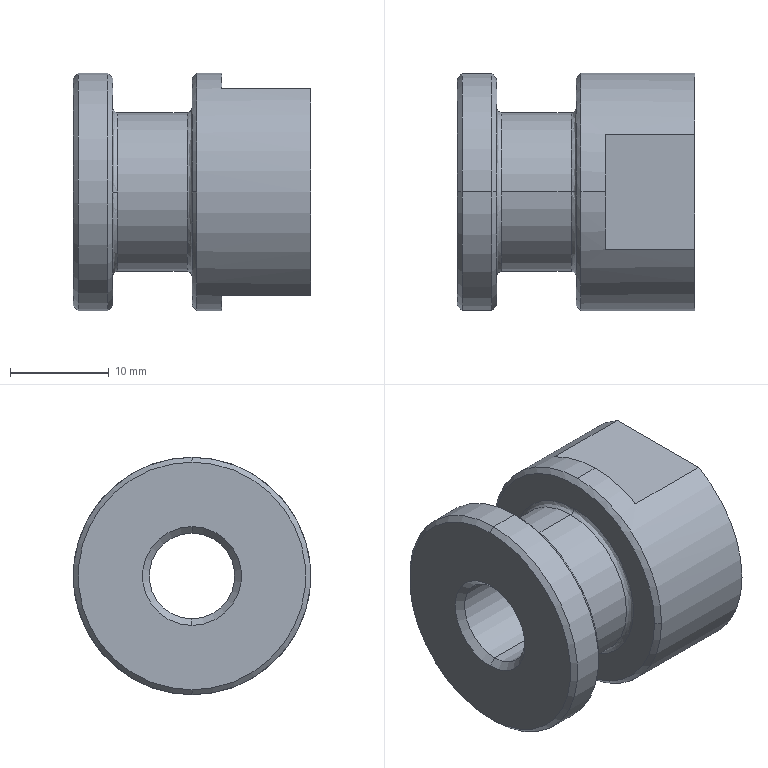Part | STEP file | FJCL10-1_25-8-a_2 | 1 solid | 28 faces | box 24 x 24 x 24 mm | volume 7197 mm3 | cylinder 8 | cone 8 | plane 8 | spline 4 | commonest cylinder face diameters 24 x4 8.647 x2 16 x2